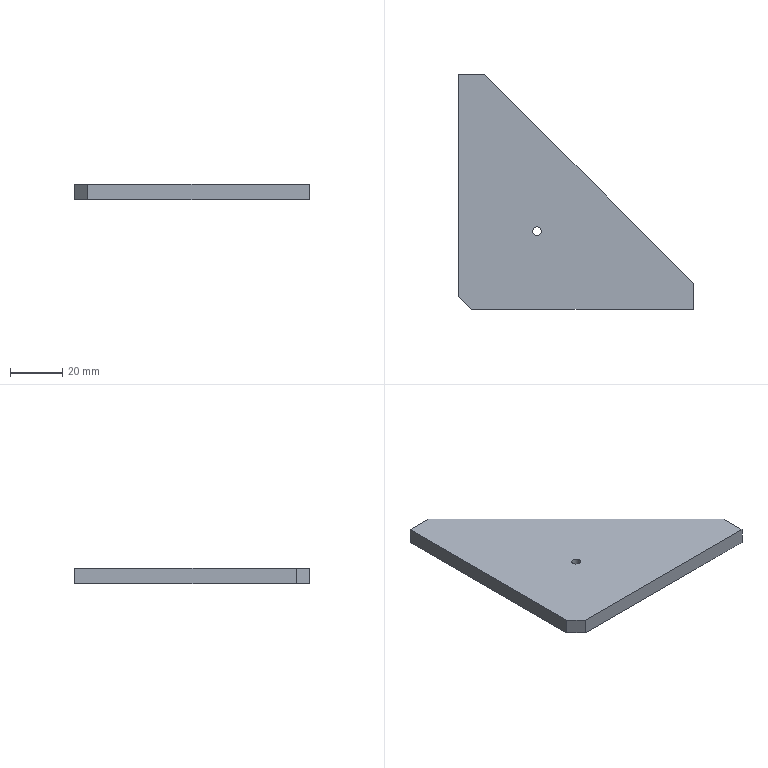Part | STEP file | 1 solid | 10 faces | box 90 x 90 x 6 mm | volume 29274 mm3 | plane 8 | cylinder 2 | commonest cylinder face diameters 3.3 x2
STEP:
#1=CARTESIAN_POINT('',(0.,0.,0.));
#2=DIRECTION('',(0.,0.,1.));
#3=DIRECTION('',(1.,0.,0.));
#4=AXIS2_PLACEMENT_3D('',#1,#2,#3);
#5=CARTESIAN_POINT('',(31.65,30.,-3.));
#6=VERTEX_POINT('',#5);
#7=CARTESIAN_POINT('',(31.65,30.,3.));
#8=VERTEX_POINT('',#7);
#9=CARTESIAN_POINT('',(31.65,30.,3.));
#10=DIRECTION('',(0.,0.,1.));
#11=VECTOR('',#10,1.);
#12=LINE('',#9,#11);
#13=CARTESIAN_POINT('',(30.,30.,3.));
#14=DIRECTION('',(0.,0.,1.));
#15=DIRECTION('',(1.,0.,0.));
#16=AXIS2_PLACEMENT_3D('',#13,#14,#15);
#17=CYLINDRICAL_SURFACE('',#16,1.65);
#18=CARTESIAN_POINT('',(6.283,0.));
#19=DIRECTION('',(0.,1.));
#20=VECTOR('',#19,1.);
#21=LINE('',#18,#20);
#22=(GEOMETRIC_REPRESENTATION_CONTEXT(2)PARAMETRIC_REPRESENTATION_CONTEXT()REPRESENTATION_CONTEXT('',''));
#23=DEFINITIONAL_REPRESENTATION('',(#21),#22);
#24=PCURVE('',#17,#23);
#25=CARTESIAN_POINT('',(30.,30.,3.));
#26=DIRECTION('',(0.,0.,1.));
#27=DIRECTION('',(1.,0.,0.));
#28=AXIS2_PLACEMENT_3D('',#25,#26,#27);
#29=CYLINDRICAL_SURFACE('',#28,1.65);
#30=CARTESIAN_POINT('',(0.,0.));
#31=DIRECTION('',(0.,1.));
#32=VECTOR('',#31,1.);
#33=LINE('',#30,#32);
#34=(GEOMETRIC_REPRESENTATION_CONTEXT(2)PARAMETRIC_REPRESENTATION_CONTEXT()REPRESENTATION_CONTEXT('',''));
#35=DEFINITIONAL_REPRESENTATION('',(#33),#34);
#36=PCURVE('',#29,#35);
#37=SURFACE_CURVE('',#12,(#24,#36),.PCURVE_S1.);
#38=EDGE_CURVE('',#6,#8,#37,.T.);
#39=ORIENTED_EDGE('',*,*,#38,.T.);
#40=CARTESIAN_POINT('',(28.35,30.,3.));
#41=VERTEX_POINT('',#40);
#42=CARTESIAN_POINT('',(30.,30.,3.));
#43=DIRECTION('',(0.,0.,1.));
#44=DIRECTION('',(1.,0.,0.));
#45=AXIS2_PLACEMENT_3D('',#42,#43,#44);
#46=CIRCLE('',#45,1.65);
#47=CARTESIAN_POINT('',(0.,0.));
#48=DIRECTION('',(1.,0.));
#49=VECTOR('',#48,1.);
#50=LINE('',#47,#49);
#51=(GEOMETRIC_REPRESENTATION_CONTEXT(2)PARAMETRIC_REPRESENTATION_CONTEXT()REPRESENTATION_CONTEXT('',''));
#52=DEFINITIONAL_REPRESENTATION('',(#50),#51);
#53=PCURVE('',#17,#52);
#54=CARTESIAN_POINT('',(0.,0.,3.));
#55=DIRECTION('',(0.,0.,-1.));
#56=DIRECTION('',(-1.,0.,0.));
#57=AXIS2_PLACEMENT_3D('',#54,#55,#56);
#58=PLANE('',#57);
#59=CARTESIAN_POINT('',(-31.65,30.));
#60=CARTESIAN_POINT('',(-31.65,32.858));
#61=CARTESIAN_POINT('',(-29.175,31.429));
#62=CARTESIAN_POINT('',(-26.7,30.));
#63=CARTESIAN_POINT('',(-29.175,28.571));
#64=CARTESIAN_POINT('',(-31.65,27.142));
#65=CARTESIAN_POINT('',(-31.65,30.));
#66=(BOUNDED_CURVE()B_SPLINE_CURVE(2,(#59,#60,#61,#62,#63,#64,#65),.UNSPECIFIED.,.T.,.F.)B_SPLINE_CURVE_WITH_KNOTS((1,2,2,2,2,1),(-2.094,0.,2.094,4.189,6.283,8.378),.UNSPECIFIED.)CURVE()GEOMETRIC_REPRESENTATION_ITEM()RATIONAL_B_SPLINE_CURVE((1.,0.5,1.,0.5,1.,0.5,1.))REPRESENTATION_ITEM(''));
#67=(GEOMETRIC_REPRESENTATION_CONTEXT(2)PARAMETRIC_REPRESENTATION_CONTEXT()REPRESENTATION_CONTEXT('',''));
#68=DEFINITIONAL_REPRESENTATION('',(#66),#67);
#69=PCURVE('',#58,#68);
#70=SURFACE_CURVE('',#46,(#53,#69),.PCURVE_S1.);
#71=EDGE_CURVE('',#41,#8,#70,.T.);
#72=ORIENTED_EDGE('',*,*,#71,.F.);
#73=CARTESIAN_POINT('',(28.35,30.,-3.));
#74=VERTEX_POINT('',#73);
#75=CARTESIAN_POINT('',(28.35,30.,3.));
#76=DIRECTION('',(0.,0.,1.));
#77=VECTOR('',#76,1.);
#78=LINE('',#75,#77);
#79=CARTESIAN_POINT('',(3.142,0.));
#80=DIRECTION('',(0.,1.));
#81=VECTOR('',#80,1.);
#82=LINE('',#79,#81);
#83=(GEOMETRIC_REPRESENTATION_CONTEXT(2)PARAMETRIC_REPRESENTATION_CONTEXT()REPRESENTATION_CONTEXT('',''));
#84=DEFINITIONAL_REPRESENTATION('',(#82),#83);
#85=PCURVE('',#17,#84);
#86=CARTESIAN_POINT('',(3.142,0.));
#87=DIRECTION('',(0.,1.));
#88=VECTOR('',#87,1.);
#89=LINE('',#86,#88);
#90=(GEOMETRIC_REPRESENTATION_CONTEXT(2)PARAMETRIC_REPRESENTATION_CONTEXT()REPRESENTATION_CONTEXT('',''));
#91=DEFINITIONAL_REPRESENTATION('',(#89),#90);
#92=PCURVE('',#29,#91);
#93=SURFACE_CURVE('',#78,(#85,#92),.PCURVE_S1.);
#94=EDGE_CURVE('',#74,#41,#93,.T.);
#95=ORIENTED_EDGE('',*,*,#94,.F.);
#96=CARTESIAN_POINT('',(30.,30.,-3.));
#97=DIRECTION('',(0.,0.,-1.));
#98=DIRECTION('',(-1.,0.,0.));
#99=AXIS2_PLACEMENT_3D('',#96,#97,#98);
#100=CIRCLE('',#99,1.65);
#101=CARTESIAN_POINT('',(9.425,-6.));
#102=DIRECTION('',(-1.,0.));
#103=VECTOR('',#102,1.);
#104=LINE('',#101,#103);
#105=(GEOMETRIC_REPRESENTATION_CONTEXT(2)PARAMETRIC_REPRESENTATION_CONTEXT()REPRESENTATION_CONTEXT('',''));
#106=DEFINITIONAL_REPRESENTATION('',(#104),#105);
#107=PCURVE('',#17,#106);
#108=CARTESIAN_POINT('',(0.,0.,-3.));
#109=DIRECTION('',(0.,0.,-1.));
#110=DIRECTION('',(-1.,0.,0.));
#111=AXIS2_PLACEMENT_3D('',#108,#109,#110);
#112=PLANE('',#111);
#113=CARTESIAN_POINT('',(-30.,30.));
#114=DIRECTION('',(1.,0.));
#115=AXIS2_PLACEMENT_2D('',#113,#114);
#116=CIRCLE('',#115,1.65);
#117=(GEOMETRIC_REPRESENTATION_CONTEXT(2)PARAMETRIC_REPRESENTATION_CONTEXT()REPRESENTATION_CONTEXT('',''));
#118=DEFINITIONAL_REPRESENTATION('',(#116),#117);
#119=PCURVE('',#112,#118);
#120=SURFACE_CURVE('',#100,(#107,#119),.PCURVE_S1.);
#121=EDGE_CURVE('',#6,#74,#120,.T.);
#122=ORIENTED_EDGE('',*,*,#121,.F.);
#123=EDGE_LOOP('',(#39,#72,#95,#122));
#124=FACE_BOUND('',#123,.F.);
#125=ADVANCED_FACE('',(#124),#17,.F.);
#126=CARTESIAN_POINT('',(90.,0.,-3.));
#127=VERTEX_POINT('',#126);
#128=CARTESIAN_POINT('',(90.,10.,-3.));
#129=VERTEX_POINT('',#128);
#130=CARTESIAN_POINT('',(90.,10.,-3.));
#131=DIRECTION('',(0.,1.,0.));
#132=VECTOR('',#131,1.);
#133=LINE('',#130,#132);
#134=CARTESIAN_POINT('',(90.,10.,3.));
#135=DIRECTION('',(-1.,0.,0.));
#136=DIRECTION('',(0.,-1.,0.));
#137=AXIS2_PLACEMENT_3D('',#134,#135,#136);
#138=PLANE('',#137);
#139=CARTESIAN_POINT('',(0.,-6.));
#140=DIRECTION('',(-1.,0.));
#141=VECTOR('',#140,1.);
#142=LINE('',#139,#141);
#143=(GEOMETRIC_REPRESENTATION_CONTEXT(2)PARAMETRIC_REPRESENTATION_CONTEXT()REPRESENTATION_CONTEXT('',''));
#144=DEFINITIONAL_REPRESENTATION('',(#142),#143);
#145=PCURVE('',#138,#144);
#146=CARTESIAN_POINT('',(-90.,10.));
#147=DIRECTION('',(0.,1.));
#148=VECTOR('',#147,1.);
#149=LINE('',#146,#148);
#150=(GEOMETRIC_REPRESENTATION_CONTEXT(2)PARAMETRIC_REPRESENTATION_CONTEXT()REPRESENTATION_CONTEXT('',''));
#151=DEFINITIONAL_REPRESENTATION('',(#149),#150);
#152=PCURVE('',#112,#151);
#153=SURFACE_CURVE('',#133,(#145,#152),.PCURVE_S1.);
#154=EDGE_CURVE('',#127,#129,#153,.T.);
#155=ORIENTED_EDGE('',*,*,#154,.T.);
#156=CARTESIAN_POINT('',(90.,10.,3.));
#157=VERTEX_POINT('',#156);
#158=CARTESIAN_POINT('',(90.,10.,3.));
#159=DIRECTION('',(0.,0.,-1.));
#160=VECTOR('',#159,1.);
#161=LINE('',#158,#160);
#162=CARTESIAN_POINT('',(0.,0.));
#163=DIRECTION('',(0.,-1.));
#164=VECTOR('',#163,1.);
#165=LINE('',#162,#164);
#166=(GEOMETRIC_REPRESENTATION_CONTEXT(2)PARAMETRIC_REPRESENTATION_CONTEXT()REPRESENTATION_CONTEXT('',''));
#167=DEFINITIONAL_REPRESENTATION('',(#165),#166);
#168=PCURVE('',#138,#167);
#169=CARTESIAN_POINT('',(10.,90.,3.));
#170=DIRECTION('',(-0.7071,-0.7071,0.));
#171=DIRECTION('',(0.7071,-0.7071,0.));
#172=AXIS2_PLACEMENT_3D('',#169,#170,#171);
#173=PLANE('',#172);
#174=CARTESIAN_POINT('',(113.137,0.));
#175=DIRECTION('',(0.,-1.));
#176=VECTOR('',#175,1.);
#177=LINE('',#174,#176);
#178=(GEOMETRIC_REPRESENTATION_CONTEXT(2)PARAMETRIC_REPRESENTATION_CONTEXT()REPRESENTATION_CONTEXT('',''));
#179=DEFINITIONAL_REPRESENTATION('',(#177),#178);
#180=PCURVE('',#173,#179);
#181=SURFACE_CURVE('',#161,(#168,#180),.PCURVE_S1.);
#182=EDGE_CURVE('',#157,#129,#181,.T.);
#183=ORIENTED_EDGE('',*,*,#182,.F.);
#184=CARTESIAN_POINT('',(90.,0.,3.));
#185=VERTEX_POINT('',#184);
#186=CARTESIAN_POINT('',(90.,10.,3.));
#187=DIRECTION('',(0.,1.,0.));
#188=VECTOR('',#187,1.);
#189=LINE('',#186,#188);
#190=CARTESIAN_POINT('',(0.,0.));
#191=DIRECTION('',(-1.,0.));
#192=VECTOR('',#191,1.);
#193=LINE('',#190,#192);
#194=(GEOMETRIC_REPRESENTATION_CONTEXT(2)PARAMETRIC_REPRESENTATION_CONTEXT()REPRESENTATION_CONTEXT('',''));
#195=DEFINITIONAL_REPRESENTATION('',(#193),#194);
#196=PCURVE('',#138,#195);
#197=CARTESIAN_POINT('',(-90.,10.));
#198=DIRECTION('',(0.,1.));
#199=VECTOR('',#198,1.);
#200=LINE('',#197,#199);
#201=(GEOMETRIC_REPRESENTATION_CONTEXT(2)PARAMETRIC_REPRESENTATION_CONTEXT()REPRESENTATION_CONTEXT('',''));
#202=DEFINITIONAL_REPRESENTATION('',(#200),#201);
#203=PCURVE('',#58,#202);
#204=SURFACE_CURVE('',#189,(#196,#203),.PCURVE_S1.);
#205=EDGE_CURVE('',#185,#157,#204,.T.);
#206=ORIENTED_EDGE('',*,*,#205,.F.);
#207=CARTESIAN_POINT('',(90.,0.,3.));
#208=DIRECTION('',(0.,0.,-1.));
#209=VECTOR('',#208,1.);
#210=LINE('',#207,#209);
#211=CARTESIAN_POINT('',(10.,0.));
#212=DIRECTION('',(0.,-1.));
#213=VECTOR('',#212,1.);
#214=LINE('',#211,#213);
#215=(GEOMETRIC_REPRESENTATION_CONTEXT(2)PARAMETRIC_REPRESENTATION_CONTEXT()REPRESENTATION_CONTEXT('',''));
#216=DEFINITIONAL_REPRESENTATION('',(#214),#215);
#217=PCURVE('',#138,#216);
#218=CARTESIAN_POINT('',(90.,0.,3.));
#219=DIRECTION('',(0.,1.,0.));
#220=DIRECTION('',(-1.,0.,0.));
#221=AXIS2_PLACEMENT_3D('',#218,#219,#220);
#222=PLANE('',#221);
#223=CARTESIAN_POINT('',(0.,0.));
#224=DIRECTION('',(0.,-1.));
#225=VECTOR('',#224,1.);
#226=LINE('',#223,#225);
#227=(GEOMETRIC_REPRESENTATION_CONTEXT(2)PARAMETRIC_REPRESENTATION_CONTEXT()REPRESENTATION_CONTEXT('',''));
#228=DEFINITIONAL_REPRESENTATION('',(#226),#227);
#229=PCURVE('',#222,#228);
#230=SURFACE_CURVE('',#210,(#217,#229),.PCURVE_S1.);
#231=EDGE_CURVE('',#185,#127,#230,.T.);
#232=ORIENTED_EDGE('',*,*,#231,.T.);
#233=EDGE_LOOP('',(#155,#183,#206,#232));
#234=FACE_BOUND('',#233,.T.);
#235=ADVANCED_FACE('',(#234),#138,.F.);
#236=CARTESIAN_POINT('',(10.,90.,-3.));
#237=VERTEX_POINT('',#236);
#238=CARTESIAN_POINT('',(10.,90.,-3.));
#239=DIRECTION('',(-0.7071,0.7071,0.));
#240=VECTOR('',#239,1.);
#241=LINE('',#238,#240);
#242=CARTESIAN_POINT('',(0.,-6.));
#243=DIRECTION('',(-1.,0.));
#244=VECTOR('',#243,1.);
#245=LINE('',#242,#244);
#246=(GEOMETRIC_REPRESENTATION_CONTEXT(2)PARAMETRIC_REPRESENTATION_CONTEXT()REPRESENTATION_CONTEXT('',''));
#247=DEFINITIONAL_REPRESENTATION('',(#245),#246);
#248=PCURVE('',#173,#247);
#249=CARTESIAN_POINT('',(-10.,90.));
#250=DIRECTION('',(0.7071,0.7071));
#251=VECTOR('',#250,1.);
#252=LINE('',#249,#251);
#253=(GEOMETRIC_REPRESENTATION_CONTEXT(2)PARAMETRIC_REPRESENTATION_CONTEXT()REPRESENTATION_CONTEXT('',''));
#254=DEFINITIONAL_REPRESENTATION('',(#252),#253);
#255=PCURVE('',#112,#254);
#256=SURFACE_CURVE('',#241,(#248,#255),.PCURVE_S1.);
#257=EDGE_CURVE('',#129,#237,#256,.T.);
#258=ORIENTED_EDGE('',*,*,#257,.T.);
#259=CARTESIAN_POINT('',(10.,90.,3.));
#260=VERTEX_POINT('',#259);
#261=CARTESIAN_POINT('',(10.,90.,3.));
#262=DIRECTION('',(0.,0.,-1.));
#263=VECTOR('',#262,1.);
#264=LINE('',#261,#263);
#265=CARTESIAN_POINT('',(0.,0.));
#266=DIRECTION('',(0.,-1.));
#267=VECTOR('',#266,1.);
#268=LINE('',#265,#267);
#269=(GEOMETRIC_REPRESENTATION_CONTEXT(2)PARAMETRIC_REPRESENTATION_CONTEXT()REPRESENTATION_CONTEXT('',''));
#270=DEFINITIONAL_REPRESENTATION('',(#268),#269);
#271=PCURVE('',#173,#270);
#272=CARTESIAN_POINT('',(0.,90.,3.));
#273=DIRECTION('',(0.,-1.,0.));
#274=DIRECTION('',(0.,0.,-1.));
#275=AXIS2_PLACEMENT_3D('',#272,#273,#274);
#276=PLANE('',#275);
#277=CARTESIAN_POINT('',(0.,10.));
#278=DIRECTION('',(1.,0.));
#279=VECTOR('',#278,1.);
#280=LINE('',#277,#279);
#281=(GEOMETRIC_REPRESENTATION_CONTEXT(2)PARAMETRIC_REPRESENTATION_CONTEXT()REPRESENTATION_CONTEXT('',''));
#282=DEFINITIONAL_REPRESENTATION('',(#280),#281);
#283=PCURVE('',#276,#282);
#284=SURFACE_CURVE('',#264,(#271,#283),.PCURVE_S1.);
#285=EDGE_CURVE('',#260,#237,#284,.T.);
#286=ORIENTED_EDGE('',*,*,#285,.F.);
#287=CARTESIAN_POINT('',(10.,90.,3.));
#288=DIRECTION('',(-0.7071,0.7071,0.));
#289=VECTOR('',#288,1.);
#290=LINE('',#287,#289);
#291=CARTESIAN_POINT('',(0.,0.));
#292=DIRECTION('',(-1.,0.));
#293=VECTOR('',#292,1.);
#294=LINE('',#291,#293);
#295=(GEOMETRIC_REPRESENTATION_CONTEXT(2)PARAMETRIC_REPRESENTATION_CONTEXT()REPRESENTATION_CONTEXT('',''));
#296=DEFINITIONAL_REPRESENTATION('',(#294),#295);
#297=PCURVE('',#173,#296);
#298=CARTESIAN_POINT('',(-10.,90.));
#299=DIRECTION('',(0.7071,0.7071));
#300=VECTOR('',#299,1.);
#301=LINE('',#298,#300);
#302=(GEOMETRIC_REPRESENTATION_CONTEXT(2)PARAMETRIC_REPRESENTATION_CONTEXT()REPRESENTATION_CONTEXT('',''));
#303=DEFINITIONAL_REPRESENTATION('',(#301),#302);
#304=PCURVE('',#58,#303);
#305=SURFACE_CURVE('',#290,(#297,#304),.PCURVE_S1.);
#306=EDGE_CURVE('',#157,#260,#305,.T.);
#307=ORIENTED_EDGE('',*,*,#306,.F.);
#308=ORIENTED_EDGE('',*,*,#182,.T.);
#309=EDGE_LOOP('',(#258,#286,#307,#308));
#310=FACE_BOUND('',#309,.T.);
#311=ADVANCED_FACE('',(#310),#173,.F.);
#312=CARTESIAN_POINT('',(0.,90.,-3.));
#313=VERTEX_POINT('',#312);
#314=CARTESIAN_POINT('',(0.,90.,-3.));
#315=DIRECTION('',(-1.,0.,0.));
#316=VECTOR('',#315,1.);
#317=LINE('',#314,#316);
#318=CARTESIAN_POINT('',(6.,0.));
#319=DIRECTION('',(0.,-1.));
#320=VECTOR('',#319,1.);
#321=LINE('',#318,#320);
#322=(GEOMETRIC_REPRESENTATION_CONTEXT(2)PARAMETRIC_REPRESENTATION_CONTEXT()REPRESENTATION_CONTEXT('',''));
#323=DEFINITIONAL_REPRESENTATION('',(#321),#322);
#324=PCURVE('',#276,#323);
#325=CARTESIAN_POINT('',(0.,90.));
#326=DIRECTION('',(1.,0.));
#327=VECTOR('',#326,1.);
#328=LINE('',#325,#327);
#329=(GEOMETRIC_REPRESENTATION_CONTEXT(2)PARAMETRIC_REPRESENTATION_CONTEXT()REPRESENTATION_CONTEXT('',''));
#330=DEFINITIONAL_REPRESENTATION('',(#328),#329);
#331=PCURVE('',#112,#330);
#332=SURFACE_CURVE('',#317,(#324,#331),.PCURVE_S1.);
#333=EDGE_CURVE('',#237,#313,#332,.T.);
#334=ORIENTED_EDGE('',*,*,#333,.T.);
#335=CARTESIAN_POINT('',(0.,90.,3.));
#336=VERTEX_POINT('',#335);
#337=CARTESIAN_POINT('',(0.,90.,3.));
#338=DIRECTION('',(0.,0.,-1.));
#339=VECTOR('',#338,1.);
#340=LINE('',#337,#339);
#341=CARTESIAN_POINT('',(0.,0.));
#342=DIRECTION('',(1.,0.));
#343=VECTOR('',#342,1.);
#344=LINE('',#341,#343);
#345=(GEOMETRIC_REPRESENTATION_CONTEXT(2)PARAMETRIC_REPRESENTATION_CONTEXT()REPRESENTATION_CONTEXT('',''));
#346=DEFINITIONAL_REPRESENTATION('',(#344),#345);
#347=PCURVE('',#276,#346);
#348=CARTESIAN_POINT('',(0.,0.,3.));
#349=DIRECTION('',(1.,0.,0.));
#350=DIRECTION('',(0.,0.,-1.));
#351=AXIS2_PLACEMENT_3D('',#348,#349,#350);
#352=PLANE('',#351);
#353=CARTESIAN_POINT('',(0.,90.));
#354=DIRECTION('',(1.,0.));
#355=VECTOR('',#354,1.);
#356=LINE('',#353,#355);
#357=(GEOMETRIC_REPRESENTATION_CONTEXT(2)PARAMETRIC_REPRESENTATION_CONTEXT()REPRESENTATION_CONTEXT('',''));
#358=DEFINITIONAL_REPRESENTATION('',(#356),#357);
#359=PCURVE('',#352,#358);
#360=SURFACE_CURVE('',#340,(#347,#359),.PCURVE_S1.);
#361=EDGE_CURVE('',#336,#313,#360,.T.);
#362=ORIENTED_EDGE('',*,*,#361,.F.);
#363=CARTESIAN_POINT('',(0.,90.,3.));
#364=DIRECTION('',(-1.,0.,0.));
#365=VECTOR('',#364,1.);
#366=LINE('',#363,#365);
#367=CARTESIAN_POINT('',(0.,0.));
#368=DIRECTION('',(0.,-1.));
#369=VECTOR('',#368,1.);
#370=LINE('',#367,#369);
#371=(GEOMETRIC_REPRESENTATION_CONTEXT(2)PARAMETRIC_REPRESENTATION_CONTEXT()REPRESENTATION_CONTEXT('',''));
#372=DEFINITIONAL_REPRESENTATION('',(#370),#371);
#373=PCURVE('',#276,#372);
#374=CARTESIAN_POINT('',(0.,90.));
#375=DIRECTION('',(1.,0.));
#376=VECTOR('',#375,1.);
#377=LINE('',#374,#376);
#378=(GEOMETRIC_REPRESENTATION_CONTEXT(2)PARAMETRIC_REPRESENTATION_CONTEXT()REPRESENTATION_CONTEXT('',''));
#379=DEFINITIONAL_REPRESENTATION('',(#377),#378);
#380=PCURVE('',#58,#379);
#381=SURFACE_CURVE('',#366,(#373,#380),.PCURVE_S1.);
#382=EDGE_CURVE('',#260,#336,#381,.T.);
#383=ORIENTED_EDGE('',*,*,#382,.F.);
#384=ORIENTED_EDGE('',*,*,#285,.T.);
#385=EDGE_LOOP('',(#334,#362,#383,#384));
#386=FACE_BOUND('',#385,.T.);
#387=ADVANCED_FACE('',(#386),#276,.F.);
#388=CARTESIAN_POINT('',(0.,5.,-3.));
#389=VERTEX_POINT('',#388);
#390=CARTESIAN_POINT('',(0.,0.,-3.));
#391=DIRECTION('',(0.,-1.,0.));
#392=VECTOR('',#391,1.);
#393=LINE('',#390,#392);
#394=CARTESIAN_POINT('',(6.,0.));
#395=DIRECTION('',(0.,-1.));
#396=VECTOR('',#395,1.);
#397=LINE('',#394,#396);
#398=(GEOMETRIC_REPRESENTATION_CONTEXT(2)PARAMETRIC_REPRESENTATION_CONTEXT()REPRESENTATION_CONTEXT('',''));
#399=DEFINITIONAL_REPRESENTATION('',(#397),#398);
#400=PCURVE('',#352,#399);
#401=CARTESIAN_POINT('',(0.,0.));
#402=DIRECTION('',(0.,-1.));
#403=VECTOR('',#402,1.);
#404=LINE('',#401,#403);
#405=(GEOMETRIC_REPRESENTATION_CONTEXT(2)PARAMETRIC_REPRESENTATION_CONTEXT()REPRESENTATION_CONTEXT('',''));
#406=DEFINITIONAL_REPRESENTATION('',(#404),#405);
#407=PCURVE('',#112,#406);
#408=SURFACE_CURVE('',#393,(#400,#407),.PCURVE_S1.);
#409=EDGE_CURVE('',#313,#389,#408,.T.);
#410=ORIENTED_EDGE('',*,*,#409,.T.);
#411=CARTESIAN_POINT('',(0.,5.,3.));
#412=VERTEX_POINT('',#411);
#413=CARTESIAN_POINT('',(0.,5.,3.));
#414=DIRECTION('',(0.,0.,1.));
#415=VECTOR('',#414,1.);
#416=LINE('',#413,#415);
#417=CARTESIAN_POINT('',(0.,5.));
#418=DIRECTION('',(-1.,0.));
#419=VECTOR('',#418,1.);
#420=LINE('',#417,#419);
#421=(GEOMETRIC_REPRESENTATION_CONTEXT(2)PARAMETRIC_REPRESENTATION_CONTEXT()REPRESENTATION_CONTEXT('',''));
#422=DEFINITIONAL_REPRESENTATION('',(#420),#421);
#423=PCURVE('',#352,#422);
#424=CARTESIAN_POINT('',(5.,0.,3.));
#425=DIRECTION('',(0.7071,0.7071,0.));
#426=DIRECTION('',(0.,0.,-1.));
#427=AXIS2_PLACEMENT_3D('',#424,#425,#426);
#428=PLANE('',#427);
#429=CARTESIAN_POINT('',(0.,7.071));
#430=DIRECTION('',(-1.,0.));
#431=VECTOR('',#430,1.);
#432=LINE('',#429,#431);
#433=(GEOMETRIC_REPRESENTATION_CONTEXT(2)PARAMETRIC_REPRESENTATION_CONTEXT()REPRESENTATION_CONTEXT('',''));
#434=DEFINITIONAL_REPRESENTATION('',(#432),#433);
#435=PCURVE('',#428,#434);
#436=SURFACE_CURVE('',#416,(#423,#435),.PCURVE_S1.);
#437=EDGE_CURVE('',#389,#412,#436,.T.);
#438=ORIENTED_EDGE('',*,*,#437,.T.);
#439=CARTESIAN_POINT('',(0.,0.,3.));
#440=DIRECTION('',(0.,-1.,0.));
#441=VECTOR('',#440,1.);
#442=LINE('',#439,#441);
#443=CARTESIAN_POINT('',(0.,0.));
#444=DIRECTION('',(0.,-1.));
#445=VECTOR('',#444,1.);
#446=LINE('',#443,#445);
#447=(GEOMETRIC_REPRESENTATION_CONTEXT(2)PARAMETRIC_REPRESENTATION_CONTEXT()REPRESENTATION_CONTEXT('',''));
#448=DEFINITIONAL_REPRESENTATION('',(#446),#447);
#449=PCURVE('',#352,#448);
#450=CARTESIAN_POINT('',(0.,0.));
#451=DIRECTION('',(0.,-1.));
#452=VECTOR('',#451,1.);
#453=LINE('',#450,#452);
#454=(GEOMETRIC_REPRESENTATION_CONTEXT(2)PARAMETRIC_REPRESENTATION_CONTEXT()REPRESENTATION_CONTEXT('',''));
#455=DEFINITIONAL_REPRESENTATION('',(#453),#454);
#456=PCURVE('',#58,#455);
#457=SURFACE_CURVE('',#442,(#449,#456),.PCURVE_S1.);
#458=EDGE_CURVE('',#336,#412,#457,.T.);
#459=ORIENTED_EDGE('',*,*,#458,.F.);
#460=ORIENTED_EDGE('',*,*,#361,.T.);
#461=EDGE_LOOP('',(#410,#438,#459,#460));
#462=FACE_BOUND('',#461,.T.);
#463=ADVANCED_FACE('',(#462),#352,.F.);
#464=CARTESIAN_POINT('',(5.,0.,3.));
#465=VERTEX_POINT('',#464);
#466=CARTESIAN_POINT('',(90.,0.,3.));
#467=DIRECTION('',(1.,0.,0.));
#468=VECTOR('',#467,1.);
#469=LINE('',#466,#468);
#470=CARTESIAN_POINT('',(0.,0.));
#471=DIRECTION('',(-1.,0.));
#472=VECTOR('',#471,1.);
#473=LINE('',#470,#472);
#474=(GEOMETRIC_REPRESENTATION_CONTEXT(2)PARAMETRIC_REPRESENTATION_CONTEXT()REPRESENTATION_CONTEXT('',''));
#475=DEFINITIONAL_REPRESENTATION('',(#473),#474);
#476=PCURVE('',#222,#475);
#477=CARTESIAN_POINT('',(-90.,0.));
#478=DIRECTION('',(-1.,0.));
#479=VECTOR('',#478,1.);
#480=LINE('',#477,#479);
#481=(GEOMETRIC_REPRESENTATION_CONTEXT(2)PARAMETRIC_REPRESENTATION_CONTEXT()REPRESENTATION_CONTEXT('',''));
#482=DEFINITIONAL_REPRESENTATION('',(#480),#481);
#483=PCURVE('',#58,#482);
#484=SURFACE_CURVE('',#469,(#476,#483),.PCURVE_S1.);
#485=EDGE_CURVE('',#465,#185,#484,.T.);
#486=ORIENTED_EDGE('',*,*,#485,.F.);
#487=CARTESIAN_POINT('',(5.,0.,-3.));
#488=VERTEX_POINT('',#487);
#489=CARTESIAN_POINT('',(5.,0.,3.));
#490=DIRECTION('',(0.,0.,-1.));
#491=VECTOR('',#490,1.);
#492=LINE('',#489,#491);
#493=CARTESIAN_POINT('',(85.,0.));
#494=DIRECTION('',(0.,-1.));
#495=VECTOR('',#494,1.);
#496=LINE('',#493,#495);
#497=(GEOMETRIC_REPRESENTATION_CONTEXT(2)PARAMETRIC_REPRESENTATION_CONTEXT()REPRESENTATION_CONTEXT('',''));
#498=DEFINITIONAL_REPRESENTATION('',(#496),#497);
#499=PCURVE('',#222,#498);
#500=CARTESIAN_POINT('',(0.,0.));
#501=DIRECTION('',(1.,0.));
#502=VECTOR('',#501,1.);
#503=LINE('',#500,#502);
#504=(GEOMETRIC_REPRESENTATION_CONTEXT(2)PARAMETRIC_REPRESENTATION_CONTEXT()REPRESENTATION_CONTEXT('',''));
#505=DEFINITIONAL_REPRESENTATION('',(#503),#504);
#506=PCURVE('',#428,#505);
#507=SURFACE_CURVE('',#492,(#499,#506),.PCURVE_S1.);
#508=EDGE_CURVE('',#465,#488,#507,.T.);
#509=ORIENTED_EDGE('',*,*,#508,.T.);
#510=CARTESIAN_POINT('',(90.,0.,-3.));
#511=DIRECTION('',(1.,0.,0.));
#512=VECTOR('',#511,1.);
#513=LINE('',#510,#512);
#514=CARTESIAN_POINT('',(0.,-6.));
#515=DIRECTION('',(-1.,0.));
#516=VECTOR('',#515,1.);
#517=LINE('',#514,#516);
#518=(GEOMETRIC_REPRESENTATION_CONTEXT(2)PARAMETRIC_REPRESENTATION_CONTEXT()REPRESENTATION_CONTEXT('',''));
#519=DEFINITIONAL_REPRESENTATION('',(#517),#518);
#520=PCURVE('',#222,#519);
#521=CARTESIAN_POINT('',(-90.,0.));
#522=DIRECTION('',(-1.,0.));
#523=VECTOR('',#522,1.);
#524=LINE('',#521,#523);
#525=(GEOMETRIC_REPRESENTATION_CONTEXT(2)PARAMETRIC_REPRESENTATION_CONTEXT()REPRESENTATION_CONTEXT('',''));
#526=DEFINITIONAL_REPRESENTATION('',(#524),#525);
#527=PCURVE('',#112,#526);
#528=SURFACE_CURVE('',#513,(#520,#527),.PCURVE_S1.);
#529=EDGE_CURVE('',#488,#127,#528,.T.);
#530=ORIENTED_EDGE('',*,*,#529,.T.);
#531=ORIENTED_EDGE('',*,*,#231,.F.);
#532=EDGE_LOOP('',(#486,#509,#530,#531));
#533=FACE_BOUND('',#532,.T.);
#534=ADVANCED_FACE('',(#533),#222,.F.);
#535=CARTESIAN_POINT('',(30.,30.,3.));
#536=DIRECTION('',(0.,0.,1.));
#537=DIRECTION('',(1.,0.,0.));
#538=AXIS2_PLACEMENT_3D('',#535,#536,#537);
#539=CIRCLE('',#538,1.65);
#540=CARTESIAN_POINT('',(-31.65,30.));
#541=CARTESIAN_POINT('',(-31.65,32.858));
#542=CARTESIAN_POINT('',(-29.175,31.429));
#543=CARTESIAN_POINT('',(-26.7,30.));
#544=CARTESIAN_POINT('',(-29.175,28.571));
#545=CARTESIAN_POINT('',(-31.65,27.142));
#546=CARTESIAN_POINT('',(-31.65,30.));
#547=(BOUNDED_CURVE()B_SPLINE_CURVE(2,(#540,#541,#542,#543,#544,#545,#546),.UNSPECIFIED.,.T.,.F.)B_SPLINE_CURVE_WITH_KNOTS((1,2,2,2,2,1),(-2.094,0.,2.094,4.189,6.283,8.378),.UNSPECIFIED.)CURVE()GEOMETRIC_REPRESENTATION_ITEM()RATIONAL_B_SPLINE_CURVE((1.,0.5,1.,0.5,1.,0.5,1.))REPRESENTATION_ITEM(''));
#548=(GEOMETRIC_REPRESENTATION_CONTEXT(2)PARAMETRIC_REPRESENTATION_CONTEXT()REPRESENTATION_CONTEXT('',''));
#549=DEFINITIONAL_REPRESENTATION('',(#547),#548);
#550=PCURVE('',#58,#549);
#551=CARTESIAN_POINT('',(0.,0.));
#552=DIRECTION('',(1.,0.));
#553=VECTOR('',#552,1.);
#554=LINE('',#551,#553);
#555=(GEOMETRIC_REPRESENTATION_CONTEXT(2)PARAMETRIC_REPRESENTATION_CONTEXT()REPRESENTATION_CONTEXT('',''));
#556=DEFINITIONAL_REPRESENTATION('',(#554),#555);
#557=PCURVE('',#29,#556);
#558=SURFACE_CURVE('',#539,(#550,#557),.PCURVE_S1.);
#559=EDGE_CURVE('',#8,#41,#558,.T.);
#560=ORIENTED_EDGE('',*,*,#559,.F.);
#561=ORIENTED_EDGE('',*,*,#71,.F.);
#562=EDGE_LOOP('',(#560,#561));
#563=FACE_BOUND('',#562,.T.);
#564=ORIENTED_EDGE('',*,*,#458,.T.);
#565=CARTESIAN_POINT('',(5.,0.,3.));
#566=DIRECTION('',(0.7071,-0.7071,0.));
#567=VECTOR('',#566,1.);
#568=LINE('',#565,#567);
#569=CARTESIAN_POINT('',(-5.,0.));
#570=DIRECTION('',(-0.7071,-0.7071));
#571=VECTOR('',#570,1.);
#572=LINE('',#569,#571);
#573=(GEOMETRIC_REPRESENTATION_CONTEXT(2)PARAMETRIC_REPRESENTATION_CONTEXT()REPRESENTATION_CONTEXT('',''));
#574=DEFINITIONAL_REPRESENTATION('',(#572),#573);
#575=PCURVE('',#58,#574);
#576=CARTESIAN_POINT('',(0.,0.));
#577=DIRECTION('',(0.,-1.));
#578=VECTOR('',#577,1.);
#579=LINE('',#576,#578);
#580=(GEOMETRIC_REPRESENTATION_CONTEXT(2)PARAMETRIC_REPRESENTATION_CONTEXT()REPRESENTATION_CONTEXT('',''));
#581=DEFINITIONAL_REPRESENTATION('',(#579),#580);
#582=PCURVE('',#428,#581);
#583=SURFACE_CURVE('',#568,(#575,#582),.PCURVE_S1.);
#584=EDGE_CURVE('',#412,#465,#583,.T.);
#585=ORIENTED_EDGE('',*,*,#584,.T.);
#586=ORIENTED_EDGE('',*,*,#485,.T.);
#587=ORIENTED_EDGE('',*,*,#205,.T.);
#588=ORIENTED_EDGE('',*,*,#306,.T.);
#589=ORIENTED_EDGE('',*,*,#382,.T.);
#590=EDGE_LOOP('',(#564,#585,#586,#587,#588,#589));
#591=FACE_BOUND('',#590,.T.);
#592=ADVANCED_FACE('',(#563,#591),#58,.F.);
#593=ORIENTED_EDGE('',*,*,#121,.F.);
#594=CARTESIAN_POINT('',(30.,30.,-3.));
#595=DIRECTION('',(0.,0.,-1.));
#596=DIRECTION('',(-1.,0.,0.));
#597=AXIS2_PLACEMENT_3D('',#594,#595,#596);
#598=CIRCLE('',#597,1.65);
#599=CARTESIAN_POINT('',(-30.,30.));
#600=DIRECTION('',(1.,0.));
#601=AXIS2_PLACEMENT_2D('',#599,#600);
#602=CIRCLE('',#601,1.65);
#603=(GEOMETRIC_REPRESENTATION_CONTEXT(2)PARAMETRIC_REPRESENTATION_CONTEXT()REPRESENTATION_CONTEXT('',''));
#604=DEFINITIONAL_REPRESENTATION('',(#602),#603);
#605=PCURVE('',#112,#604);
#606=CARTESIAN_POINT('',(3.142,-6.));
#607=DIRECTION('',(-1.,0.));
#608=VECTOR('',#607,1.);
#609=LINE('',#606,#608);
#610=(GEOMETRIC_REPRESENTATION_CONTEXT(2)PARAMETRIC_REPRESENTATION_CONTEXT()REPRESENTATION_CONTEXT('',''));
#611=DEFINITIONAL_REPRESENTATION('',(#609),#610);
#612=PCURVE('',#29,#611);
#613=SURFACE_CURVE('',#598,(#605,#612),.PCURVE_S1.);
#614=EDGE_CURVE('',#74,#6,#613,.T.);
#615=ORIENTED_EDGE('',*,*,#614,.F.);
#616=EDGE_LOOP('',(#593,#615));
#617=FACE_BOUND('',#616,.T.);
#618=ORIENTED_EDGE('',*,*,#529,.F.);
#619=CARTESIAN_POINT('',(2.5,2.5,-3.));
#620=DIRECTION('',(-0.7071,0.7071,0.));
#621=VECTOR('',#620,1.);
#622=LINE('',#619,#621);
#623=CARTESIAN_POINT('',(-2.5,2.5));
#624=DIRECTION('',(0.7071,0.7071));
#625=VECTOR('',#624,1.);
#626=LINE('',#623,#625);
#627=(GEOMETRIC_REPRESENTATION_CONTEXT(2)PARAMETRIC_REPRESENTATION_CONTEXT()REPRESENTATION_CONTEXT('',''));
#628=DEFINITIONAL_REPRESENTATION('',(#626),#627);
#629=PCURVE('',#112,#628);
#630=CARTESIAN_POINT('',(6.,3.536));
#631=DIRECTION('',(0.,1.));
#632=VECTOR('',#631,1.);
#633=LINE('',#630,#632);
#634=(GEOMETRIC_REPRESENTATION_CONTEXT(2)PARAMETRIC_REPRESENTATION_CONTEXT()REPRESENTATION_CONTEXT('',''));
#635=DEFINITIONAL_REPRESENTATION('',(#633),#634);
#636=PCURVE('',#428,#635);
#637=SURFACE_CURVE('',#622,(#629,#636),.PCURVE_S1.);
#638=EDGE_CURVE('',#488,#389,#637,.T.);
#639=ORIENTED_EDGE('',*,*,#638,.T.);
#640=ORIENTED_EDGE('',*,*,#409,.F.);
#641=ORIENTED_EDGE('',*,*,#333,.F.);
#642=ORIENTED_EDGE('',*,*,#257,.F.);
#643=ORIENTED_EDGE('',*,*,#154,.F.);
#644=EDGE_LOOP('',(#618,#639,#640,#641,#642,#643));
#645=FACE_BOUND('',#644,.T.);
#646=ADVANCED_FACE('',(#617,#645),#112,.T.);
#647=ORIENTED_EDGE('',*,*,#584,.F.);
#648=ORIENTED_EDGE('',*,*,#437,.F.);
#649=ORIENTED_EDGE('',*,*,#638,.F.);
#650=ORIENTED_EDGE('',*,*,#508,.F.);
#651=EDGE_LOOP('',(#647,#648,#649,#650));
#652=FACE_BOUND('',#651,.T.);
#653=ADVANCED_FACE('',(#652),#428,.F.);
#654=ORIENTED_EDGE('',*,*,#559,.F.);
#655=ORIENTED_EDGE('',*,*,#38,.F.);
#656=ORIENTED_EDGE('',*,*,#614,.F.);
#657=ORIENTED_EDGE('',*,*,#94,.T.);
#658=EDGE_LOOP('',(#654,#655,#656,#657));
#659=FACE_BOUND('',#658,.F.);
#660=ADVANCED_FACE('',(#659),#29,.F.);
#661=CLOSED_SHELL('',(#125,#235,#311,#387,#463,#534,#592,#646,#653,#660));
#662=MANIFOLD_SOLID_BREP('',#661);
#663=(LENGTH_UNIT()NAMED_UNIT(*)SI_UNIT(.MILLI.,.METRE.));
#664=UNCERTAINTY_MEASURE_WITH_UNIT(LENGTH_MEASURE(0.0000001),#663,'','');
#665=(NAMED_UNIT(*)PLANE_ANGLE_UNIT()SI_UNIT($,.RADIAN.));
#666=(NAMED_UNIT(*)SI_UNIT($,.STERADIAN.)SOLID_ANGLE_UNIT());
#667=(GEOMETRIC_REPRESENTATION_CONTEXT(3)GLOBAL_UNCERTAINTY_ASSIGNED_CONTEXT((#664))GLOBAL_UNIT_ASSIGNED_CONTEXT((#663,#665,#666))REPRESENTATION_CONTEXT('',''));
#668=ADVANCED_BREP_SHAPE_REPRESENTATION('',(#4,#662),#667);